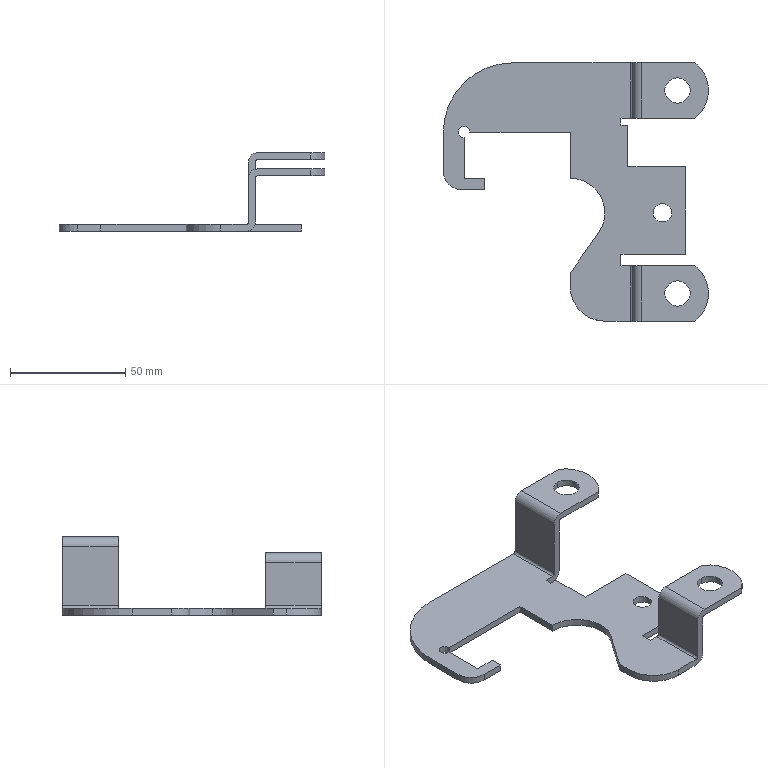Part | STEP file | 8XS123010 | 1 solid | 52 faces | box 115 x 112 x 34 mm | volume 22620 mm3 | plane 30 | cylinder 22 | commonest cylinder face diameters 8 x6 30 x5 2 x4 11 x4 5 x1 16 x1